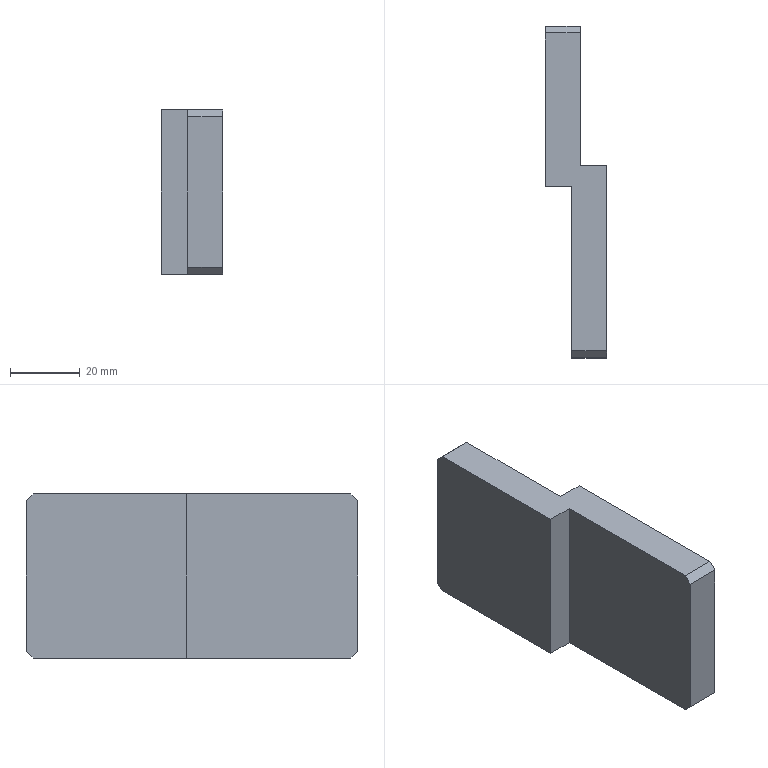Part | STEP file | PN_0041 | 1 solid | 14 faces | box 17.5 x 95 x 47 mm | volume 46685 mm3 | plane 14
STEP:
#1=CARTESIAN_POINT('',(0.,0.,0.));
#2=DIRECTION('',(0.,0.,1.));
#3=DIRECTION('',(1.,0.,0.));
#4=AXIS2_PLACEMENT_3D('',#1,#2,#3);
#5=CARTESIAN_POINT('',(10.,95.,45.));
#6=VERTEX_POINT('',#5);
#7=CARTESIAN_POINT('',(10.,95.,2.));
#8=VERTEX_POINT('',#7);
#9=CARTESIAN_POINT('',(10.,95.,47.));
#10=DIRECTION('',(0.,0.,-1.));
#11=VECTOR('',#10,1.);
#12=LINE('',#9,#11);
#13=CARTESIAN_POINT('',(0.,95.,47.));
#14=DIRECTION('',(0.,-1.,0.));
#15=DIRECTION('',(0.,0.,-1.));
#16=AXIS2_PLACEMENT_3D('',#13,#14,#15);
#17=PLANE('',#16);
#18=CARTESIAN_POINT('',(0.,10.));
#19=DIRECTION('',(1.,0.));
#20=VECTOR('',#19,1.);
#21=LINE('',#18,#20);
#22=(GEOMETRIC_REPRESENTATION_CONTEXT(2)PARAMETRIC_REPRESENTATION_CONTEXT()REPRESENTATION_CONTEXT('',''));
#23=DEFINITIONAL_REPRESENTATION('',(#21),#22);
#24=PCURVE('',#17,#23);
#25=CARTESIAN_POINT('',(10.,95.,47.));
#26=DIRECTION('',(-1.,0.,0.));
#27=DIRECTION('',(0.,-1.,0.));
#28=AXIS2_PLACEMENT_3D('',#25,#26,#27);
#29=PLANE('',#28);
#30=CARTESIAN_POINT('',(0.,0.));
#31=DIRECTION('',(0.,-1.));
#32=VECTOR('',#31,1.);
#33=LINE('',#30,#32);
#34=(GEOMETRIC_REPRESENTATION_CONTEXT(2)PARAMETRIC_REPRESENTATION_CONTEXT()REPRESENTATION_CONTEXT('',''));
#35=DEFINITIONAL_REPRESENTATION('',(#33),#34);
#36=PCURVE('',#29,#35);
#37=SURFACE_CURVE('',#12,(#24,#36),.PCURVE_S1.);
#38=EDGE_CURVE('',#6,#8,#37,.T.);
#39=ORIENTED_EDGE('',*,*,#38,.T.);
#40=CARTESIAN_POINT('',(0.,95.,2.));
#41=VERTEX_POINT('',#40);
#42=CARTESIAN_POINT('',(0.,95.,2.));
#43=DIRECTION('',(-1.,0.,0.));
#44=VECTOR('',#43,1.);
#45=LINE('',#42,#44);
#46=CARTESIAN_POINT('',(45.,0.));
#47=DIRECTION('',(0.,-1.));
#48=VECTOR('',#47,1.);
#49=LINE('',#46,#48);
#50=(GEOMETRIC_REPRESENTATION_CONTEXT(2)PARAMETRIC_REPRESENTATION_CONTEXT()REPRESENTATION_CONTEXT('',''));
#51=DEFINITIONAL_REPRESENTATION('',(#49),#50);
#52=PCURVE('',#17,#51);
#53=CARTESIAN_POINT('',(0.,95.,2.));
#54=DIRECTION('',(0.,0.7071,-0.7071));
#55=DIRECTION('',(0.,0.7071,0.7071));
#56=AXIS2_PLACEMENT_3D('',#53,#54,#55);
#57=PLANE('',#56);
#58=CARTESIAN_POINT('',(0.,0.));
#59=DIRECTION('',(0.,-1.));
#60=VECTOR('',#59,1.);
#61=LINE('',#58,#60);
#62=(GEOMETRIC_REPRESENTATION_CONTEXT(2)PARAMETRIC_REPRESENTATION_CONTEXT()REPRESENTATION_CONTEXT('',''));
#63=DEFINITIONAL_REPRESENTATION('',(#61),#62);
#64=PCURVE('',#57,#63);
#65=SURFACE_CURVE('',#45,(#52,#64),.PCURVE_S1.);
#66=EDGE_CURVE('',#8,#41,#65,.T.);
#67=ORIENTED_EDGE('',*,*,#66,.T.);
#68=CARTESIAN_POINT('',(0.,95.,45.));
#69=VERTEX_POINT('',#68);
#70=CARTESIAN_POINT('',(0.,95.,47.));
#71=DIRECTION('',(0.,0.,-1.));
#72=VECTOR('',#71,1.);
#73=LINE('',#70,#72);
#74=CARTESIAN_POINT('',(0.,0.));
#75=DIRECTION('',(1.,0.));
#76=VECTOR('',#75,1.);
#77=LINE('',#74,#76);
#78=(GEOMETRIC_REPRESENTATION_CONTEXT(2)PARAMETRIC_REPRESENTATION_CONTEXT()REPRESENTATION_CONTEXT('',''));
#79=DEFINITIONAL_REPRESENTATION('',(#77),#78);
#80=PCURVE('',#17,#79);
#81=CARTESIAN_POINT('',(0.,49.,47.));
#82=DIRECTION('',(1.,0.,0.));
#83=DIRECTION('',(0.,0.,-1.));
#84=AXIS2_PLACEMENT_3D('',#81,#82,#83);
#85=PLANE('',#84);
#86=CARTESIAN_POINT('',(0.,46.));
#87=DIRECTION('',(1.,0.));
#88=VECTOR('',#87,1.);
#89=LINE('',#86,#88);
#90=(GEOMETRIC_REPRESENTATION_CONTEXT(2)PARAMETRIC_REPRESENTATION_CONTEXT()REPRESENTATION_CONTEXT('',''));
#91=DEFINITIONAL_REPRESENTATION('',(#89),#90);
#92=PCURVE('',#85,#91);
#93=SURFACE_CURVE('',#73,(#80,#92),.PCURVE_S1.);
#94=EDGE_CURVE('',#69,#41,#93,.T.);
#95=ORIENTED_EDGE('',*,*,#94,.F.);
#96=CARTESIAN_POINT('',(0.,95.,45.));
#97=DIRECTION('',(1.,0.,0.));
#98=VECTOR('',#97,1.);
#99=LINE('',#96,#98);
#100=CARTESIAN_POINT('',(2.,0.));
#101=DIRECTION('',(0.,1.));
#102=VECTOR('',#101,1.);
#103=LINE('',#100,#102);
#104=(GEOMETRIC_REPRESENTATION_CONTEXT(2)PARAMETRIC_REPRESENTATION_CONTEXT()REPRESENTATION_CONTEXT('',''));
#105=DEFINITIONAL_REPRESENTATION('',(#103),#104);
#106=PCURVE('',#17,#105);
#107=CARTESIAN_POINT('',(10.,93.,47.));
#108=DIRECTION('',(0.,-0.7071,-0.7071));
#109=DIRECTION('',(0.,0.7071,-0.7071));
#110=AXIS2_PLACEMENT_3D('',#107,#108,#109);
#111=PLANE('',#110);
#112=CARTESIAN_POINT('',(2.828,-10.));
#113=DIRECTION('',(0.,1.));
#114=VECTOR('',#113,1.);
#115=LINE('',#112,#114);
#116=(GEOMETRIC_REPRESENTATION_CONTEXT(2)PARAMETRIC_REPRESENTATION_CONTEXT()REPRESENTATION_CONTEXT('',''));
#117=DEFINITIONAL_REPRESENTATION('',(#115),#116);
#118=PCURVE('',#111,#117);
#119=SURFACE_CURVE('',#99,(#106,#118),.PCURVE_S1.);
#120=EDGE_CURVE('',#69,#6,#119,.T.);
#121=ORIENTED_EDGE('',*,*,#120,.T.);
#122=EDGE_LOOP('',(#39,#67,#95,#121));
#123=FACE_BOUND('',#122,.T.);
#124=ADVANCED_FACE('',(#123),#17,.F.);
#125=ORIENTED_EDGE('',*,*,#94,.T.);
#126=CARTESIAN_POINT('',(0.,93.,0.));
#127=VERTEX_POINT('',#126);
#128=CARTESIAN_POINT('',(0.,95.,2.));
#129=DIRECTION('',(0.,-0.7071,-0.7071));
#130=VECTOR('',#129,1.);
#131=LINE('',#128,#130);
#132=CARTESIAN_POINT('',(45.,46.));
#133=DIRECTION('',(0.7071,-0.7071));
#134=VECTOR('',#133,1.);
#135=LINE('',#132,#134);
#136=(GEOMETRIC_REPRESENTATION_CONTEXT(2)PARAMETRIC_REPRESENTATION_CONTEXT()REPRESENTATION_CONTEXT('',''));
#137=DEFINITIONAL_REPRESENTATION('',(#135),#136);
#138=PCURVE('',#85,#137);
#139=CARTESIAN_POINT('',(0.,0.));
#140=DIRECTION('',(-1.,0.));
#141=VECTOR('',#140,1.);
#142=LINE('',#139,#141);
#143=(GEOMETRIC_REPRESENTATION_CONTEXT(2)PARAMETRIC_REPRESENTATION_CONTEXT()REPRESENTATION_CONTEXT('',''));
#144=DEFINITIONAL_REPRESENTATION('',(#142),#143);
#145=PCURVE('',#57,#144);
#146=SURFACE_CURVE('',#131,(#138,#145),.PCURVE_S1.);
#147=EDGE_CURVE('',#41,#127,#146,.T.);
#148=ORIENTED_EDGE('',*,*,#147,.T.);
#149=CARTESIAN_POINT('',(0.,49.,0.));
#150=VERTEX_POINT('',#149);
#151=CARTESIAN_POINT('',(0.,49.,0.));
#152=DIRECTION('',(0.,-1.,0.));
#153=VECTOR('',#152,1.);
#154=LINE('',#151,#153);
#155=CARTESIAN_POINT('',(47.,0.));
#156=DIRECTION('',(0.,-1.));
#157=VECTOR('',#156,1.);
#158=LINE('',#155,#157);
#159=(GEOMETRIC_REPRESENTATION_CONTEXT(2)PARAMETRIC_REPRESENTATION_CONTEXT()REPRESENTATION_CONTEXT('',''));
#160=DEFINITIONAL_REPRESENTATION('',(#158),#159);
#161=PCURVE('',#85,#160);
#162=CARTESIAN_POINT('',(10.,95.,0.));
#163=DIRECTION('',(0.,0.,-1.));
#164=DIRECTION('',(-1.,0.,0.));
#165=AXIS2_PLACEMENT_3D('',#162,#163,#164);
#166=PLANE('',#165);
#167=CARTESIAN_POINT('',(10.,-46.));
#168=DIRECTION('',(0.,-1.));
#169=VECTOR('',#168,1.);
#170=LINE('',#167,#169);
#171=(GEOMETRIC_REPRESENTATION_CONTEXT(2)PARAMETRIC_REPRESENTATION_CONTEXT()REPRESENTATION_CONTEXT('',''));
#172=DEFINITIONAL_REPRESENTATION('',(#170),#171);
#173=PCURVE('',#166,#172);
#174=SURFACE_CURVE('',#154,(#161,#173),.PCURVE_S1.);
#175=EDGE_CURVE('',#127,#150,#174,.T.);
#176=ORIENTED_EDGE('',*,*,#175,.T.);
#177=CARTESIAN_POINT('',(0.,49.,47.));
#178=VERTEX_POINT('',#177);
#179=CARTESIAN_POINT('',(0.,49.,47.));
#180=DIRECTION('',(0.,0.,-1.));
#181=VECTOR('',#180,1.);
#182=LINE('',#179,#181);
#183=CARTESIAN_POINT('',(0.,0.));
#184=DIRECTION('',(1.,0.));
#185=VECTOR('',#184,1.);
#186=LINE('',#183,#185);
#187=(GEOMETRIC_REPRESENTATION_CONTEXT(2)PARAMETRIC_REPRESENTATION_CONTEXT()REPRESENTATION_CONTEXT('',''));
#188=DEFINITIONAL_REPRESENTATION('',(#186),#187);
#189=PCURVE('',#85,#188);
#190=CARTESIAN_POINT('',(0.,49.,47.));
#191=DIRECTION('',(0.,1.,0.));
#192=DIRECTION('',(0.,0.,1.));
#193=AXIS2_PLACEMENT_3D('',#190,#191,#192);
#194=PLANE('',#193);
#195=CARTESIAN_POINT('',(0.,0.));
#196=DIRECTION('',(-1.,0.));
#197=VECTOR('',#196,1.);
#198=LINE('',#195,#197);
#199=(GEOMETRIC_REPRESENTATION_CONTEXT(2)PARAMETRIC_REPRESENTATION_CONTEXT()REPRESENTATION_CONTEXT('',''));
#200=DEFINITIONAL_REPRESENTATION('',(#198),#199);
#201=PCURVE('',#194,#200);
#202=SURFACE_CURVE('',#182,(#189,#201),.PCURVE_S1.);
#203=EDGE_CURVE('',#178,#150,#202,.T.);
#204=ORIENTED_EDGE('',*,*,#203,.F.);
#205=CARTESIAN_POINT('',(0.,93.,47.));
#206=VERTEX_POINT('',#205);
#207=CARTESIAN_POINT('',(0.,49.,47.));
#208=DIRECTION('',(0.,-1.,0.));
#209=VECTOR('',#208,1.);
#210=LINE('',#207,#209);
#211=CARTESIAN_POINT('',(0.,0.));
#212=DIRECTION('',(0.,-1.));
#213=VECTOR('',#212,1.);
#214=LINE('',#211,#213);
#215=(GEOMETRIC_REPRESENTATION_CONTEXT(2)PARAMETRIC_REPRESENTATION_CONTEXT()REPRESENTATION_CONTEXT('',''));
#216=DEFINITIONAL_REPRESENTATION('',(#214),#215);
#217=PCURVE('',#85,#216);
#218=CARTESIAN_POINT('',(10.,95.,47.));
#219=DIRECTION('',(0.,0.,-1.));
#220=DIRECTION('',(-1.,0.,0.));
#221=AXIS2_PLACEMENT_3D('',#218,#219,#220);
#222=PLANE('',#221);
#223=CARTESIAN_POINT('',(10.,-46.));
#224=DIRECTION('',(0.,-1.));
#225=VECTOR('',#224,1.);
#226=LINE('',#223,#225);
#227=(GEOMETRIC_REPRESENTATION_CONTEXT(2)PARAMETRIC_REPRESENTATION_CONTEXT()REPRESENTATION_CONTEXT('',''));
#228=DEFINITIONAL_REPRESENTATION('',(#226),#227);
#229=PCURVE('',#222,#228);
#230=SURFACE_CURVE('',#210,(#217,#229),.PCURVE_S1.);
#231=EDGE_CURVE('',#206,#178,#230,.T.);
#232=ORIENTED_EDGE('',*,*,#231,.F.);
#233=CARTESIAN_POINT('',(0.,93.,47.));
#234=DIRECTION('',(0.,0.7071,-0.7071));
#235=VECTOR('',#234,1.);
#236=LINE('',#233,#235);
#237=CARTESIAN_POINT('',(0.,44.));
#238=DIRECTION('',(0.7071,0.7071));
#239=VECTOR('',#238,1.);
#240=LINE('',#237,#239);
#241=(GEOMETRIC_REPRESENTATION_CONTEXT(2)PARAMETRIC_REPRESENTATION_CONTEXT()REPRESENTATION_CONTEXT('',''));
#242=DEFINITIONAL_REPRESENTATION('',(#240),#241);
#243=PCURVE('',#85,#242);
#244=CARTESIAN_POINT('',(0.,-10.));
#245=DIRECTION('',(1.,0.));
#246=VECTOR('',#245,1.);
#247=LINE('',#244,#246);
#248=(GEOMETRIC_REPRESENTATION_CONTEXT(2)PARAMETRIC_REPRESENTATION_CONTEXT()REPRESENTATION_CONTEXT('',''));
#249=DEFINITIONAL_REPRESENTATION('',(#247),#248);
#250=PCURVE('',#111,#249);
#251=SURFACE_CURVE('',#236,(#243,#250),.PCURVE_S1.);
#252=EDGE_CURVE('',#206,#69,#251,.T.);
#253=ORIENTED_EDGE('',*,*,#252,.T.);
#254=EDGE_LOOP('',(#125,#148,#176,#204,#232,#253));
#255=FACE_BOUND('',#254,.T.);
#256=ADVANCED_FACE('',(#255),#85,.F.);
#257=CARTESIAN_POINT('',(7.5,49.,0.));
#258=VERTEX_POINT('',#257);
#259=CARTESIAN_POINT('',(0.,49.,0.));
#260=DIRECTION('',(1.,0.,0.));
#261=VECTOR('',#260,1.);
#262=LINE('',#259,#261);
#263=CARTESIAN_POINT('',(-47.,0.));
#264=DIRECTION('',(0.,1.));
#265=VECTOR('',#264,1.);
#266=LINE('',#263,#265);
#267=(GEOMETRIC_REPRESENTATION_CONTEXT(2)PARAMETRIC_REPRESENTATION_CONTEXT()REPRESENTATION_CONTEXT('',''));
#268=DEFINITIONAL_REPRESENTATION('',(#266),#267);
#269=PCURVE('',#194,#268);
#270=CARTESIAN_POINT('',(10.,-46.));
#271=DIRECTION('',(-1.,0.));
#272=VECTOR('',#271,1.);
#273=LINE('',#270,#272);
#274=(GEOMETRIC_REPRESENTATION_CONTEXT(2)PARAMETRIC_REPRESENTATION_CONTEXT()REPRESENTATION_CONTEXT('',''));
#275=DEFINITIONAL_REPRESENTATION('',(#273),#274);
#276=PCURVE('',#166,#275);
#277=SURFACE_CURVE('',#262,(#269,#276),.PCURVE_S1.);
#278=EDGE_CURVE('',#150,#258,#277,.T.);
#279=ORIENTED_EDGE('',*,*,#278,.T.);
#280=CARTESIAN_POINT('',(7.5,49.,47.));
#281=VERTEX_POINT('',#280);
#282=CARTESIAN_POINT('',(7.5,49.,47.));
#283=DIRECTION('',(0.,0.,-1.));
#284=VECTOR('',#283,1.);
#285=LINE('',#282,#284);
#286=CARTESIAN_POINT('',(0.,7.5));
#287=DIRECTION('',(-1.,0.));
#288=VECTOR('',#287,1.);
#289=LINE('',#286,#288);
#290=(GEOMETRIC_REPRESENTATION_CONTEXT(2)PARAMETRIC_REPRESENTATION_CONTEXT()REPRESENTATION_CONTEXT('',''));
#291=DEFINITIONAL_REPRESENTATION('',(#289),#290);
#292=PCURVE('',#194,#291);
#293=CARTESIAN_POINT('',(7.5,49.,47.));
#294=DIRECTION('',(1.,0.,0.));
#295=DIRECTION('',(0.,1.,0.));
#296=AXIS2_PLACEMENT_3D('',#293,#294,#295);
#297=PLANE('',#296);
#298=CARTESIAN_POINT('',(0.,0.));
#299=DIRECTION('',(0.,-1.));
#300=VECTOR('',#299,1.);
#301=LINE('',#298,#300);
#302=(GEOMETRIC_REPRESENTATION_CONTEXT(2)PARAMETRIC_REPRESENTATION_CONTEXT()REPRESENTATION_CONTEXT('',''));
#303=DEFINITIONAL_REPRESENTATION('',(#301),#302);
#304=PCURVE('',#297,#303);
#305=SURFACE_CURVE('',#285,(#292,#304),.PCURVE_S1.);
#306=EDGE_CURVE('',#281,#258,#305,.T.);
#307=ORIENTED_EDGE('',*,*,#306,.F.);
#308=CARTESIAN_POINT('',(0.,49.,47.));
#309=DIRECTION('',(1.,0.,0.));
#310=VECTOR('',#309,1.);
#311=LINE('',#308,#310);
#312=CARTESIAN_POINT('',(0.,0.));
#313=DIRECTION('',(0.,1.));
#314=VECTOR('',#313,1.);
#315=LINE('',#312,#314);
#316=(GEOMETRIC_REPRESENTATION_CONTEXT(2)PARAMETRIC_REPRESENTATION_CONTEXT()REPRESENTATION_CONTEXT('',''));
#317=DEFINITIONAL_REPRESENTATION('',(#315),#316);
#318=PCURVE('',#194,#317);
#319=CARTESIAN_POINT('',(10.,-46.));
#320=DIRECTION('',(-1.,0.));
#321=VECTOR('',#320,1.);
#322=LINE('',#319,#321);
#323=(GEOMETRIC_REPRESENTATION_CONTEXT(2)PARAMETRIC_REPRESENTATION_CONTEXT()REPRESENTATION_CONTEXT('',''));
#324=DEFINITIONAL_REPRESENTATION('',(#322),#323);
#325=PCURVE('',#222,#324);
#326=SURFACE_CURVE('',#311,(#318,#325),.PCURVE_S1.);
#327=EDGE_CURVE('',#178,#281,#326,.T.);
#328=ORIENTED_EDGE('',*,*,#327,.F.);
#329=ORIENTED_EDGE('',*,*,#203,.T.);
#330=EDGE_LOOP('',(#279,#307,#328,#329));
#331=FACE_BOUND('',#330,.T.);
#332=ADVANCED_FACE('',(#331),#194,.F.);
#333=CARTESIAN_POINT('',(7.5,2.,0.));
#334=VERTEX_POINT('',#333);
#335=CARTESIAN_POINT('',(7.5,49.,0.));
#336=DIRECTION('',(0.,-1.,0.));
#337=VECTOR('',#336,1.);
#338=LINE('',#335,#337);
#339=CARTESIAN_POINT('',(0.,-47.));
#340=DIRECTION('',(-1.,0.));
#341=VECTOR('',#340,1.);
#342=LINE('',#339,#341);
#343=(GEOMETRIC_REPRESENTATION_CONTEXT(2)PARAMETRIC_REPRESENTATION_CONTEXT()REPRESENTATION_CONTEXT('',''));
#344=DEFINITIONAL_REPRESENTATION('',(#342),#343);
#345=PCURVE('',#297,#344);
#346=CARTESIAN_POINT('',(2.5,-46.));
#347=DIRECTION('',(0.,-1.));
#348=VECTOR('',#347,1.);
#349=LINE('',#346,#348);
#350=(GEOMETRIC_REPRESENTATION_CONTEXT(2)PARAMETRIC_REPRESENTATION_CONTEXT()REPRESENTATION_CONTEXT('',''));
#351=DEFINITIONAL_REPRESENTATION('',(#349),#350);
#352=PCURVE('',#166,#351);
#353=SURFACE_CURVE('',#338,(#345,#352),.PCURVE_S1.);
#354=EDGE_CURVE('',#258,#334,#353,.T.);
#355=ORIENTED_EDGE('',*,*,#354,.T.);
#356=CARTESIAN_POINT('',(7.5,0.,2.));
#357=VERTEX_POINT('',#356);
#358=CARTESIAN_POINT('',(7.5,0.,2.));
#359=DIRECTION('',(0.,-0.7071,0.7071));
#360=VECTOR('',#359,1.);
#361=LINE('',#358,#360);
#362=CARTESIAN_POINT('',(-49.,-45.));
#363=DIRECTION('',(-0.7071,0.7071));
#364=VECTOR('',#363,1.);
#365=LINE('',#362,#364);
#366=(GEOMETRIC_REPRESENTATION_CONTEXT(2)PARAMETRIC_REPRESENTATION_CONTEXT()REPRESENTATION_CONTEXT('',''));
#367=DEFINITIONAL_REPRESENTATION('',(#365),#366);
#368=PCURVE('',#297,#367);
#369=CARTESIAN_POINT('',(7.5,0.,2.));
#370=DIRECTION('',(0.,-0.7071,-0.7071));
#371=DIRECTION('',(0.,0.7071,-0.7071));
#372=AXIS2_PLACEMENT_3D('',#369,#370,#371);
#373=PLANE('',#372);
#374=CARTESIAN_POINT('',(0.,0.));
#375=DIRECTION('',(-1.,0.));
#376=VECTOR('',#375,1.);
#377=LINE('',#374,#376);
#378=(GEOMETRIC_REPRESENTATION_CONTEXT(2)PARAMETRIC_REPRESENTATION_CONTEXT()REPRESENTATION_CONTEXT('',''));
#379=DEFINITIONAL_REPRESENTATION('',(#377),#378);
#380=PCURVE('',#373,#379);
#381=SURFACE_CURVE('',#361,(#368,#380),.PCURVE_S1.);
#382=EDGE_CURVE('',#334,#357,#381,.T.);
#383=ORIENTED_EDGE('',*,*,#382,.T.);
#384=CARTESIAN_POINT('',(7.5,0.,45.));
#385=VERTEX_POINT('',#384);
#386=CARTESIAN_POINT('',(7.5,0.,47.));
#387=DIRECTION('',(0.,0.,-1.));
#388=VECTOR('',#387,1.);
#389=LINE('',#386,#388);
#390=CARTESIAN_POINT('',(-49.,0.));
#391=DIRECTION('',(0.,-1.));
#392=VECTOR('',#391,1.);
#393=LINE('',#390,#392);
#394=(GEOMETRIC_REPRESENTATION_CONTEXT(2)PARAMETRIC_REPRESENTATION_CONTEXT()REPRESENTATION_CONTEXT('',''));
#395=DEFINITIONAL_REPRESENTATION('',(#393),#394);
#396=PCURVE('',#297,#395);
#397=CARTESIAN_POINT('',(7.5,0.,47.));
#398=DIRECTION('',(0.,1.,0.));
#399=DIRECTION('',(0.,0.,1.));
#400=AXIS2_PLACEMENT_3D('',#397,#398,#399);
#401=PLANE('',#400);
#402=CARTESIAN_POINT('',(0.,0.));
#403=DIRECTION('',(-1.,0.));
#404=VECTOR('',#403,1.);
#405=LINE('',#402,#404);
#406=(GEOMETRIC_REPRESENTATION_CONTEXT(2)PARAMETRIC_REPRESENTATION_CONTEXT()REPRESENTATION_CONTEXT('',''));
#407=DEFINITIONAL_REPRESENTATION('',(#405),#406);
#408=PCURVE('',#401,#407);
#409=SURFACE_CURVE('',#389,(#396,#408),.PCURVE_S1.);
#410=EDGE_CURVE('',#385,#357,#409,.T.);
#411=ORIENTED_EDGE('',*,*,#410,.F.);
#412=CARTESIAN_POINT('',(7.5,2.,47.));
#413=VERTEX_POINT('',#412);
#414=CARTESIAN_POINT('',(7.5,2.,47.));
#415=DIRECTION('',(0.,0.7071,0.7071));
#416=VECTOR('',#415,1.);
#417=LINE('',#414,#416);
#418=CARTESIAN_POINT('',(-47.,0.));
#419=DIRECTION('',(0.7071,0.7071));
#420=VECTOR('',#419,1.);
#421=LINE('',#418,#420);
#422=(GEOMETRIC_REPRESENTATION_CONTEXT(2)PARAMETRIC_REPRESENTATION_CONTEXT()REPRESENTATION_CONTEXT('',''));
#423=DEFINITIONAL_REPRESENTATION('',(#421),#422);
#424=PCURVE('',#297,#423);
#425=CARTESIAN_POINT('',(10.,2.,47.));
#426=DIRECTION('',(0.,0.7071,-0.7071));
#427=DIRECTION('',(0.,0.7071,0.7071));
#428=AXIS2_PLACEMENT_3D('',#425,#426,#427);
#429=PLANE('',#428);
#430=CARTESIAN_POINT('',(0.,-2.5));
#431=DIRECTION('',(1.,0.));
#432=VECTOR('',#431,1.);
#433=LINE('',#430,#432);
#434=(GEOMETRIC_REPRESENTATION_CONTEXT(2)PARAMETRIC_REPRESENTATION_CONTEXT()REPRESENTATION_CONTEXT('',''));
#435=DEFINITIONAL_REPRESENTATION('',(#433),#434);
#436=PCURVE('',#429,#435);
#437=SURFACE_CURVE('',#417,(#424,#436),.PCURVE_S1.);
#438=EDGE_CURVE('',#385,#413,#437,.T.);
#439=ORIENTED_EDGE('',*,*,#438,.T.);
#440=CARTESIAN_POINT('',(7.5,49.,47.));
#441=DIRECTION('',(0.,-1.,0.));
#442=VECTOR('',#441,1.);
#443=LINE('',#440,#442);
#444=CARTESIAN_POINT('',(0.,0.));
#445=DIRECTION('',(-1.,0.));
#446=VECTOR('',#445,1.);
#447=LINE('',#444,#446);
#448=(GEOMETRIC_REPRESENTATION_CONTEXT(2)PARAMETRIC_REPRESENTATION_CONTEXT()REPRESENTATION_CONTEXT('',''));
#449=DEFINITIONAL_REPRESENTATION('',(#447),#448);
#450=PCURVE('',#297,#449);
#451=CARTESIAN_POINT('',(2.5,-46.));
#452=DIRECTION('',(0.,-1.));
#453=VECTOR('',#452,1.);
#454=LINE('',#451,#453);
#455=(GEOMETRIC_REPRESENTATION_CONTEXT(2)PARAMETRIC_REPRESENTATION_CONTEXT()REPRESENTATION_CONTEXT('',''));
#456=DEFINITIONAL_REPRESENTATION('',(#454),#455);
#457=PCURVE('',#222,#456);
#458=SURFACE_CURVE('',#443,(#450,#457),.PCURVE_S1.);
#459=EDGE_CURVE('',#281,#413,#458,.T.);
#460=ORIENTED_EDGE('',*,*,#459,.F.);
#461=ORIENTED_EDGE('',*,*,#306,.T.);
#462=EDGE_LOOP('',(#355,#383,#411,#439,#460,#461));
#463=FACE_BOUND('',#462,.T.);
#464=ADVANCED_FACE('',(#463),#297,.F.);
#465=ORIENTED_EDGE('',*,*,#410,.T.);
#466=CARTESIAN_POINT('',(17.5,0.,2.));
#467=VERTEX_POINT('',#466);
#468=CARTESIAN_POINT('',(17.5,0.,2.));
#469=DIRECTION('',(1.,0.,0.));
#470=VECTOR('',#469,1.);
#471=LINE('',#468,#470);
#472=CARTESIAN_POINT('',(-45.,10.));
#473=DIRECTION('',(0.,1.));
#474=VECTOR('',#473,1.);
#475=LINE('',#472,#474);
#476=(GEOMETRIC_REPRESENTATION_CONTEXT(2)PARAMETRIC_REPRESENTATION_CONTEXT()REPRESENTATION_CONTEXT('',''));
#477=DEFINITIONAL_REPRESENTATION('',(#475),#476);
#478=PCURVE('',#401,#477);
#479=CARTESIAN_POINT('',(0.,10.));
#480=DIRECTION('',(0.,1.));
#481=VECTOR('',#480,1.);
#482=LINE('',#479,#481);
#483=(GEOMETRIC_REPRESENTATION_CONTEXT(2)PARAMETRIC_REPRESENTATION_CONTEXT()REPRESENTATION_CONTEXT('',''));
#484=DEFINITIONAL_REPRESENTATION('',(#482),#483);
#485=PCURVE('',#373,#484);
#486=SURFACE_CURVE('',#471,(#478,#485),.PCURVE_S1.);
#487=EDGE_CURVE('',#357,#467,#486,.T.);
#488=ORIENTED_EDGE('',*,*,#487,.T.);
#489=CARTESIAN_POINT('',(17.5,0.,45.));
#490=VERTEX_POINT('',#489);
#491=CARTESIAN_POINT('',(17.5,0.,47.));
#492=DIRECTION('',(0.,0.,-1.));
#493=VECTOR('',#492,1.);
#494=LINE('',#491,#493);
#495=CARTESIAN_POINT('',(0.,10.));
#496=DIRECTION('',(-1.,0.));
#497=VECTOR('',#496,1.);
#498=LINE('',#495,#497);
#499=(GEOMETRIC_REPRESENTATION_CONTEXT(2)PARAMETRIC_REPRESENTATION_CONTEXT()REPRESENTATION_CONTEXT('',''));
#500=DEFINITIONAL_REPRESENTATION('',(#498),#499);
#501=PCURVE('',#401,#500);
#502=CARTESIAN_POINT('',(17.5,0.,47.));
#503=DIRECTION('',(-1.,0.,0.));
#504=DIRECTION('',(0.,0.,1.));
#505=AXIS2_PLACEMENT_3D('',#502,#503,#504);
#506=PLANE('',#505);
#507=CARTESIAN_POINT('',(0.,0.));
#508=DIRECTION('',(-1.,0.));
#509=VECTOR('',#508,1.);
#510=LINE('',#507,#509);
#511=(GEOMETRIC_REPRESENTATION_CONTEXT(2)PARAMETRIC_REPRESENTATION_CONTEXT()REPRESENTATION_CONTEXT('',''));
#512=DEFINITIONAL_REPRESENTATION('',(#510),#511);
#513=PCURVE('',#506,#512);
#514=SURFACE_CURVE('',#494,(#501,#513),.PCURVE_S1.);
#515=EDGE_CURVE('',#490,#467,#514,.T.);
#516=ORIENTED_EDGE('',*,*,#515,.F.);
#517=CARTESIAN_POINT('',(7.5,0.,45.));
#518=DIRECTION('',(-1.,0.,0.));
#519=VECTOR('',#518,1.);
#520=LINE('',#517,#519);
#521=CARTESIAN_POINT('',(-2.,0.));
#522=DIRECTION('',(0.,-1.));
#523=VECTOR('',#522,1.);
#524=LINE('',#521,#523);
#525=(GEOMETRIC_REPRESENTATION_CONTEXT(2)PARAMETRIC_REPRESENTATION_CONTEXT()REPRESENTATION_CONTEXT('',''));
#526=DEFINITIONAL_REPRESENTATION('',(#524),#525);
#527=PCURVE('',#401,#526);
#528=CARTESIAN_POINT('',(-2.828,-2.5));
#529=DIRECTION('',(0.,-1.));
#530=VECTOR('',#529,1.);
#531=LINE('',#528,#530);
#532=(GEOMETRIC_REPRESENTATION_CONTEXT(2)PARAMETRIC_REPRESENTATION_CONTEXT()REPRESENTATION_CONTEXT('',''));
#533=DEFINITIONAL_REPRESENTATION('',(#531),#532);
#534=PCURVE('',#429,#533);
#535=SURFACE_CURVE('',#520,(#527,#534),.PCURVE_S1.);
#536=EDGE_CURVE('',#490,#385,#535,.T.);
#537=ORIENTED_EDGE('',*,*,#536,.T.);
#538=EDGE_LOOP('',(#465,#488,#516,#537));
#539=FACE_BOUND('',#538,.T.);
#540=ADVANCED_FACE('',(#539),#401,.F.);
#541=ORIENTED_EDGE('',*,*,#515,.T.);
#542=CARTESIAN_POINT('',(17.5,2.,0.));
#543=VERTEX_POINT('',#542);
#544=CARTESIAN_POINT('',(17.5,0.,2.));
#545=DIRECTION('',(0.,0.7071,-0.7071));
#546=VECTOR('',#545,1.);
#547=LINE('',#544,#546);
#548=CARTESIAN_POINT('',(-45.,0.));
#549=DIRECTION('',(-0.7071,0.7071));
#550=VECTOR('',#549,1.);
#551=LINE('',#548,#550);
#552=(GEOMETRIC_REPRESENTATION_CONTEXT(2)PARAMETRIC_REPRESENTATION_CONTEXT()REPRESENTATION_CONTEXT('',''));
#553=DEFINITIONAL_REPRESENTATION('',(#551),#552);
#554=PCURVE('',#506,#553);
#555=CARTESIAN_POINT('',(0.,10.));
#556=DIRECTION('',(1.,0.));
#557=VECTOR('',#556,1.);
#558=LINE('',#555,#557);
#559=(GEOMETRIC_REPRESENTATION_CONTEXT(2)PARAMETRIC_REPRESENTATION_CONTEXT()REPRESENTATION_CONTEXT('',''));
#560=DEFINITIONAL_REPRESENTATION('',(#558),#559);
#561=PCURVE('',#373,#560);
#562=SURFACE_CURVE('',#547,(#554,#561),.PCURVE_S1.);
#563=EDGE_CURVE('',#467,#543,#562,.T.);
#564=ORIENTED_EDGE('',*,*,#563,.T.);
#565=CARTESIAN_POINT('',(17.5,55.,0.));
#566=VERTEX_POINT('',#565);
#567=CARTESIAN_POINT('',(17.5,0.,0.));
#568=DIRECTION('',(0.,1.,0.));
#569=VECTOR('',#568,1.);
#570=LINE('',#567,#569);
#571=CARTESIAN_POINT('',(-47.,0.));
#572=DIRECTION('',(0.,1.));
#573=VECTOR('',#572,1.);
#574=LINE('',#571,#573);
#575=(GEOMETRIC_REPRESENTATION_CONTEXT(2)PARAMETRIC_REPRESENTATION_CONTEXT()REPRESENTATION_CONTEXT('',''));
#576=DEFINITIONAL_REPRESENTATION('',(#574),#575);
#577=PCURVE('',#506,#576);
#578=CARTESIAN_POINT('',(-7.5,-95.));
#579=DIRECTION('',(0.,1.));
#580=VECTOR('',#579,1.);
#581=LINE('',#578,#580);
#582=(GEOMETRIC_REPRESENTATION_CONTEXT(2)PARAMETRIC_REPRESENTATION_CONTEXT()REPRESENTATION_CONTEXT('',''));
#583=DEFINITIONAL_REPRESENTATION('',(#581),#582);
#584=PCURVE('',#166,#583);
#585=SURFACE_CURVE('',#570,(#577,#584),.PCURVE_S1.);
#586=EDGE_CURVE('',#543,#566,#585,.T.);
#587=ORIENTED_EDGE('',*,*,#586,.T.);
#588=CARTESIAN_POINT('',(17.5,55.,47.));
#589=VERTEX_POINT('',#588);
#590=CARTESIAN_POINT('',(17.5,55.,47.));
#591=DIRECTION('',(0.,0.,-1.));
#592=VECTOR('',#591,1.);
#593=LINE('',#590,#592);
#594=CARTESIAN_POINT('',(0.,55.));
#595=DIRECTION('',(-1.,0.));
#596=VECTOR('',#595,1.);
#597=LINE('',#594,#596);
#598=(GEOMETRIC_REPRESENTATION_CONTEXT(2)PARAMETRIC_REPRESENTATION_CONTEXT()REPRESENTATION_CONTEXT('',''));
#599=DEFINITIONAL_REPRESENTATION('',(#597),#598);
#600=PCURVE('',#506,#599);
#601=CARTESIAN_POINT('',(10.,55.,47.));
#602=DIRECTION('',(0.,-1.,0.));
#603=DIRECTION('',(0.,0.,-1.));
#604=AXIS2_PLACEMENT_3D('',#601,#602,#603);
#605=PLANE('',#604);
#606=CARTESIAN_POINT('',(0.,7.5));
#607=DIRECTION('',(1.,0.));
#608=VECTOR('',#607,1.);
#609=LINE('',#606,#608);
#610=(GEOMETRIC_REPRESENTATION_CONTEXT(2)PARAMETRIC_REPRESENTATION_CONTEXT()REPRESENTATION_CONTEXT('',''));
#611=DEFINITIONAL_REPRESENTATION('',(#609),#610);
#612=PCURVE('',#605,#611);
#613=SURFACE_CURVE('',#593,(#600,#612),.PCURVE_S1.);
#614=EDGE_CURVE('',#589,#566,#613,.T.);
#615=ORIENTED_EDGE('',*,*,#614,.F.);
#616=CARTESIAN_POINT('',(17.5,2.,47.));
#617=VERTEX_POINT('',#616);
#618=CARTESIAN_POINT('',(17.5,0.,47.));
#619=DIRECTION('',(0.,1.,0.));
#620=VECTOR('',#619,1.);
#621=LINE('',#618,#620);
#622=CARTESIAN_POINT('',(0.,0.));
#623=DIRECTION('',(0.,1.));
#624=VECTOR('',#623,1.);
#625=LINE('',#622,#624);
#626=(GEOMETRIC_REPRESENTATION_CONTEXT(2)PARAMETRIC_REPRESENTATION_CONTEXT()REPRESENTATION_CONTEXT('',''));
#627=DEFINITIONAL_REPRESENTATION('',(#625),#626);
#628=PCURVE('',#506,#627);
#629=CARTESIAN_POINT('',(-7.5,-95.));
#630=DIRECTION('',(0.,1.));
#631=VECTOR('',#630,1.);
#632=LINE('',#629,#631);
#633=(GEOMETRIC_REPRESENTATION_CONTEXT(2)PARAMETRIC_REPRESENTATION_CONTEXT()REPRESENTATION_CONTEXT('',''));
#634=DEFINITIONAL_REPRESENTATION('',(#632),#633);
#635=PCURVE('',#222,#634);
#636=SURFACE_CURVE('',#621,(#628,#635),.PCURVE_S1.);
#637=EDGE_CURVE('',#617,#589,#636,.T.);
#638=ORIENTED_EDGE('',*,*,#637,.F.);
#639=CARTESIAN_POINT('',(17.5,2.,47.));
#640=DIRECTION('',(0.,-0.7071,-0.7071));
#641=VECTOR('',#640,1.);
#642=LINE('',#639,#641);
#643=CARTESIAN_POINT('',(0.,2.));
#644=DIRECTION('',(-0.7071,-0.7071));
#645=VECTOR('',#644,1.);
#646=LINE('',#643,#645);
#647=(GEOMETRIC_REPRESENTATION_CONTEXT(2)PARAMETRIC_REPRESENTATION_CONTEXT()REPRESENTATION_CONTEXT('',''));
#648=DEFINITIONAL_REPRESENTATION('',(#646),#647);
#649=PCURVE('',#506,#648);
#650=CARTESIAN_POINT('',(0.,7.5));
#651=DIRECTION('',(-1.,0.));
#652=VECTOR('',#651,1.);
#653=LINE('',#650,#652);
#654=(GEOMETRIC_REPRESENTATION_CONTEXT(2)PARAMETRIC_REPRESENTATION_CONTEXT()REPRESENTATION_CONTEXT('',''));
#655=DEFINITIONAL_REPRESENTATION('',(#653),#654);
#656=PCURVE('',#429,#655);
#657=SURFACE_CURVE('',#642,(#649,#656),.PCURVE_S1.);
#658=EDGE_CURVE('',#617,#490,#657,.T.);
#659=ORIENTED_EDGE('',*,*,#658,.T.);
#660=EDGE_LOOP('',(#541,#564,#587,#615,#638,#659));
#661=FACE_BOUND('',#660,.T.);
#662=ADVANCED_FACE('',(#661),#506,.F.);
#663=CARTESIAN_POINT('',(10.,55.,0.));
#664=VERTEX_POINT('',#663);
#665=CARTESIAN_POINT('',(10.,55.,0.));
#666=DIRECTION('',(-1.,0.,0.));
#667=VECTOR('',#666,1.);
#668=LINE('',#665,#667);
#669=CARTESIAN_POINT('',(47.,0.));
#670=DIRECTION('',(0.,-1.));
#671=VECTOR('',#670,1.);
#672=LINE('',#669,#671);
#673=(GEOMETRIC_REPRESENTATION_CONTEXT(2)PARAMETRIC_REPRESENTATION_CONTEXT()REPRESENTATION_CONTEXT('',''));
#674=DEFINITIONAL_REPRESENTATION('',(#672),#673);
#675=PCURVE('',#605,#674);
#676=CARTESIAN_POINT('',(0.,-40.));
#677=DIRECTION('',(1.,0.));
#678=VECTOR('',#677,1.);
#679=LINE('',#676,#678);
#680=(GEOMETRIC_REPRESENTATION_CONTEXT(2)PARAMETRIC_REPRESENTATION_CONTEXT()REPRESENTATION_CONTEXT('',''));
#681=DEFINITIONAL_REPRESENTATION('',(#679),#680);
#682=PCURVE('',#166,#681);
#683=SURFACE_CURVE('',#668,(#675,#682),.PCURVE_S1.);
#684=EDGE_CURVE('',#566,#664,#683,.T.);
#685=ORIENTED_EDGE('',*,*,#684,.T.);
#686=CARTESIAN_POINT('',(10.,55.,47.));
#687=VERTEX_POINT('',#686);
#688=CARTESIAN_POINT('',(10.,55.,47.));
#689=DIRECTION('',(0.,0.,-1.));
#690=VECTOR('',#689,1.);
#691=LINE('',#688,#690);
#692=CARTESIAN_POINT('',(0.,0.));
#693=DIRECTION('',(1.,0.));
#694=VECTOR('',#693,1.);
#695=LINE('',#692,#694);
#696=(GEOMETRIC_REPRESENTATION_CONTEXT(2)PARAMETRIC_REPRESENTATION_CONTEXT()REPRESENTATION_CONTEXT('',''));
#697=DEFINITIONAL_REPRESENTATION('',(#695),#696);
#698=PCURVE('',#605,#697);
#699=CARTESIAN_POINT('',(40.,0.));
#700=DIRECTION('',(0.,-1.));
#701=VECTOR('',#700,1.);
#702=LINE('',#699,#701);
#703=(GEOMETRIC_REPRESENTATION_CONTEXT(2)PARAMETRIC_REPRESENTATION_CONTEXT()REPRESENTATION_CONTEXT('',''));
#704=DEFINITIONAL_REPRESENTATION('',(#702),#703);
#705=PCURVE('',#29,#704);
#706=SURFACE_CURVE('',#691,(#698,#705),.PCURVE_S1.);
#707=EDGE_CURVE('',#687,#664,#706,.T.);
#708=ORIENTED_EDGE('',*,*,#707,.F.);
#709=CARTESIAN_POINT('',(10.,55.,47.));
#710=DIRECTION('',(-1.,0.,0.));
#711=VECTOR('',#710,1.);
#712=LINE('',#709,#711);
#713=CARTESIAN_POINT('',(0.,0.));
#714=DIRECTION('',(0.,-1.));
#715=VECTOR('',#714,1.);
#716=LINE('',#713,#715);
#717=(GEOMETRIC_REPRESENTATION_CONTEXT(2)PARAMETRIC_REPRESENTATION_CONTEXT()REPRESENTATION_CONTEXT('',''));
#718=DEFINITIONAL_REPRESENTATION('',(#716),#717);
#719=PCURVE('',#605,#718);
#720=CARTESIAN_POINT('',(0.,-40.));
#721=DIRECTION('',(1.,0.));
#722=VECTOR('',#721,1.);
#723=LINE('',#720,#722);
#724=(GEOMETRIC_REPRESENTATION_CONTEXT(2)PARAMETRIC_REPRESENTATION_CONTEXT()REPRESENTATION_CONTEXT('',''));
#725=DEFINITIONAL_REPRESENTATION('',(#723),#724);
#726=PCURVE('',#222,#725);
#727=SURFACE_CURVE('',#712,(#719,#726),.PCURVE_S1.);
#728=EDGE_CURVE('',#589,#687,#727,.T.);
#729=ORIENTED_EDGE('',*,*,#728,.F.);
#730=ORIENTED_EDGE('',*,*,#614,.T.);
#731=EDGE_LOOP('',(#685,#708,#729,#730));
#732=FACE_BOUND('',#731,.T.);
#733=ADVANCED_FACE('',(#732),#605,.F.);
#734=CARTESIAN_POINT('',(10.,93.,0.));
#735=VERTEX_POINT('',#734);
#736=CARTESIAN_POINT('',(10.,95.,0.));
#737=DIRECTION('',(0.,1.,0.));
#738=VECTOR('',#737,1.);
#739=LINE('',#736,#738);
#740=CARTESIAN_POINT('',(0.,-47.));
#741=DIRECTION('',(-1.,0.));
#742=VECTOR('',#741,1.);
#743=LINE('',#740,#742);
#744=(GEOMETRIC_REPRESENTATION_CONTEXT(2)PARAMETRIC_REPRESENTATION_CONTEXT()REPRESENTATION_CONTEXT('',''));
#745=DEFINITIONAL_REPRESENTATION('',(#743),#744);
#746=PCURVE('',#29,#745);
#747=CARTESIAN_POINT('',(0.,0.));
#748=DIRECTION('',(0.,1.));
#749=VECTOR('',#748,1.);
#750=LINE('',#747,#749);
#751=(GEOMETRIC_REPRESENTATION_CONTEXT(2)PARAMETRIC_REPRESENTATION_CONTEXT()REPRESENTATION_CONTEXT('',''));
#752=DEFINITIONAL_REPRESENTATION('',(#750),#751);
#753=PCURVE('',#166,#752);
#754=SURFACE_CURVE('',#739,(#746,#753),.PCURVE_S1.);
#755=EDGE_CURVE('',#664,#735,#754,.T.);
#756=ORIENTED_EDGE('',*,*,#755,.T.);
#757=CARTESIAN_POINT('',(10.,95.,2.));
#758=DIRECTION('',(0.,0.7071,0.7071));
#759=VECTOR('',#758,1.);
#760=LINE('',#757,#759);
#761=CARTESIAN_POINT('',(0.,-45.));
#762=DIRECTION('',(-0.7071,0.7071));
#763=VECTOR('',#762,1.);
#764=LINE('',#761,#763);
#765=(GEOMETRIC_REPRESENTATION_CONTEXT(2)PARAMETRIC_REPRESENTATION_CONTEXT()REPRESENTATION_CONTEXT('',''));
#766=DEFINITIONAL_REPRESENTATION('',(#764),#765);
#767=PCURVE('',#29,#766);
#768=CARTESIAN_POINT('',(0.,10.));
#769=DIRECTION('',(1.,0.));
#770=VECTOR('',#769,1.);
#771=LINE('',#768,#770);
#772=(GEOMETRIC_REPRESENTATION_CONTEXT(2)PARAMETRIC_REPRESENTATION_CONTEXT()REPRESENTATION_CONTEXT('',''));
#773=DEFINITIONAL_REPRESENTATION('',(#771),#772);
#774=PCURVE('',#57,#773);
#775=SURFACE_CURVE('',#760,(#767,#774),.PCURVE_S1.);
#776=EDGE_CURVE('',#735,#8,#775,.T.);
#777=ORIENTED_EDGE('',*,*,#776,.T.);
#778=ORIENTED_EDGE('',*,*,#38,.F.);
#779=CARTESIAN_POINT('',(10.,93.,47.));
#780=VERTEX_POINT('',#779);
#781=CARTESIAN_POINT('',(10.,93.,47.));
#782=DIRECTION('',(0.,-0.7071,0.7071));
#783=VECTOR('',#782,1.);
#784=LINE('',#781,#783);
#785=CARTESIAN_POINT('',(2.,0.));
#786=DIRECTION('',(0.7071,0.7071));
#787=VECTOR('',#786,1.);
#788=LINE('',#785,#787);
#789=(GEOMETRIC_REPRESENTATION_CONTEXT(2)PARAMETRIC_REPRESENTATION_CONTEXT()REPRESENTATION_CONTEXT('',''));
#790=DEFINITIONAL_REPRESENTATION('',(#788),#789);
#791=PCURVE('',#29,#790);
#792=CARTESIAN_POINT('',(0.,0.));
#793=DIRECTION('',(-1.,0.));
#794=VECTOR('',#793,1.);
#795=LINE('',#792,#794);
#796=(GEOMETRIC_REPRESENTATION_CONTEXT(2)PARAMETRIC_REPRESENTATION_CONTEXT()REPRESENTATION_CONTEXT('',''));
#797=DEFINITIONAL_REPRESENTATION('',(#795),#796);
#798=PCURVE('',#111,#797);
#799=SURFACE_CURVE('',#784,(#791,#798),.PCURVE_S1.);
#800=EDGE_CURVE('',#6,#780,#799,.T.);
#801=ORIENTED_EDGE('',*,*,#800,.T.);
#802=CARTESIAN_POINT('',(10.,95.,47.));
#803=DIRECTION('',(0.,1.,0.));
#804=VECTOR('',#803,1.);
#805=LINE('',#802,#804);
#806=CARTESIAN_POINT('',(0.,0.));
#807=DIRECTION('',(-1.,0.));
#808=VECTOR('',#807,1.);
#809=LINE('',#806,#808);
#810=(GEOMETRIC_REPRESENTATION_CONTEXT(2)PARAMETRIC_REPRESENTATION_CONTEXT()REPRESENTATION_CONTEXT('',''));
#811=DEFINITIONAL_REPRESENTATION('',(#809),#810);
#812=PCURVE('',#29,#811);
#813=CARTESIAN_POINT('',(0.,0.));
#814=DIRECTION('',(0.,1.));
#815=VECTOR('',#814,1.);
#816=LINE('',#813,#815);
#817=(GEOMETRIC_REPRESENTATION_CONTEXT(2)PARAMETRIC_REPRESENTATION_CONTEXT()REPRESENTATION_CONTEXT('',''));
#818=DEFINITIONAL_REPRESENTATION('',(#816),#817);
#819=PCURVE('',#222,#818);
#820=SURFACE_CURVE('',#805,(#812,#819),.PCURVE_S1.);
#821=EDGE_CURVE('',#687,#780,#820,.T.);
#822=ORIENTED_EDGE('',*,*,#821,.F.);
#823=ORIENTED_EDGE('',*,*,#707,.T.);
#824=EDGE_LOOP('',(#756,#777,#778,#801,#822,#823));
#825=FACE_BOUND('',#824,.T.);
#826=ADVANCED_FACE('',(#825),#29,.F.);
#827=ORIENTED_EDGE('',*,*,#459,.T.);
#828=CARTESIAN_POINT('',(10.,2.,47.));
#829=DIRECTION('',(1.,0.,0.));
#830=VECTOR('',#829,1.);
#831=LINE('',#828,#830);
#832=CARTESIAN_POINT('',(0.,-93.));
#833=DIRECTION('',(-1.,0.));
#834=VECTOR('',#833,1.);
#835=LINE('',#832,#834);
#836=(GEOMETRIC_REPRESENTATION_CONTEXT(2)PARAMETRIC_REPRESENTATION_CONTEXT()REPRESENTATION_CONTEXT('',''));
#837=DEFINITIONAL_REPRESENTATION('',(#835),#836);
#838=PCURVE('',#222,#837);
#839=CARTESIAN_POINT('',(0.,0.));
#840=DIRECTION('',(0.,1.));
#841=VECTOR('',#840,1.);
#842=LINE('',#839,#841);
#843=(GEOMETRIC_REPRESENTATION_CONTEXT(2)PARAMETRIC_REPRESENTATION_CONTEXT()REPRESENTATION_CONTEXT('',''));
#844=DEFINITIONAL_REPRESENTATION('',(#842),#843);
#845=PCURVE('',#429,#844);
#846=SURFACE_CURVE('',#831,(#838,#845),.PCURVE_S1.);
#847=EDGE_CURVE('',#413,#617,#846,.T.);
#848=ORIENTED_EDGE('',*,*,#847,.T.);
#849=ORIENTED_EDGE('',*,*,#637,.T.);
#850=ORIENTED_EDGE('',*,*,#728,.T.);
#851=ORIENTED_EDGE('',*,*,#821,.T.);
#852=CARTESIAN_POINT('',(10.,93.,47.));
#853=DIRECTION('',(-1.,0.,0.));
#854=VECTOR('',#853,1.);
#855=LINE('',#852,#854);
#856=CARTESIAN_POINT('',(0.,-2.));
#857=DIRECTION('',(1.,0.));
#858=VECTOR('',#857,1.);
#859=LINE('',#856,#858);
#860=(GEOMETRIC_REPRESENTATION_CONTEXT(2)PARAMETRIC_REPRESENTATION_CONTEXT()REPRESENTATION_CONTEXT('',''));
#861=DEFINITIONAL_REPRESENTATION('',(#859),#860);
#862=PCURVE('',#222,#861);
#863=CARTESIAN_POINT('',(0.,0.));
#864=DIRECTION('',(0.,-1.));
#865=VECTOR('',#864,1.);
#866=LINE('',#863,#865);
#867=(GEOMETRIC_REPRESENTATION_CONTEXT(2)PARAMETRIC_REPRESENTATION_CONTEXT()REPRESENTATION_CONTEXT('',''));
#868=DEFINITIONAL_REPRESENTATION('',(#866),#867);
#869=PCURVE('',#111,#868);
#870=SURFACE_CURVE('',#855,(#862,#869),.PCURVE_S1.);
#871=EDGE_CURVE('',#780,#206,#870,.T.);
#872=ORIENTED_EDGE('',*,*,#871,.T.);
#873=ORIENTED_EDGE('',*,*,#231,.T.);
#874=ORIENTED_EDGE('',*,*,#327,.T.);
#875=EDGE_LOOP('',(#827,#848,#849,#850,#851,#872,#873,#874));
#876=FACE_BOUND('',#875,.T.);
#877=ADVANCED_FACE('',(#876),#222,.F.);
#878=ORIENTED_EDGE('',*,*,#586,.F.);
#879=CARTESIAN_POINT('',(7.5,2.,0.));
#880=DIRECTION('',(-1.,0.,0.));
#881=VECTOR('',#880,1.);
#882=LINE('',#879,#881);
#883=CARTESIAN_POINT('',(2.5,-93.));
#884=DIRECTION('',(1.,0.));
#885=VECTOR('',#884,1.);
#886=LINE('',#883,#885);
#887=(GEOMETRIC_REPRESENTATION_CONTEXT(2)PARAMETRIC_REPRESENTATION_CONTEXT()REPRESENTATION_CONTEXT('',''));
#888=DEFINITIONAL_REPRESENTATION('',(#886),#887);
#889=PCURVE('',#166,#888);
#890=CARTESIAN_POINT('',(2.828,0.));
#891=DIRECTION('',(0.,-1.));
#892=VECTOR('',#891,1.);
#893=LINE('',#890,#892);
#894=(GEOMETRIC_REPRESENTATION_CONTEXT(2)PARAMETRIC_REPRESENTATION_CONTEXT()REPRESENTATION_CONTEXT('',''));
#895=DEFINITIONAL_REPRESENTATION('',(#893),#894);
#896=PCURVE('',#373,#895);
#897=SURFACE_CURVE('',#882,(#889,#896),.PCURVE_S1.);
#898=EDGE_CURVE('',#543,#334,#897,.T.);
#899=ORIENTED_EDGE('',*,*,#898,.T.);
#900=ORIENTED_EDGE('',*,*,#354,.F.);
#901=ORIENTED_EDGE('',*,*,#278,.F.);
#902=ORIENTED_EDGE('',*,*,#175,.F.);
#903=CARTESIAN_POINT('',(10.,93.,0.));
#904=DIRECTION('',(1.,0.,0.));
#905=VECTOR('',#904,1.);
#906=LINE('',#903,#905);
#907=CARTESIAN_POINT('',(0.,-2.));
#908=DIRECTION('',(-1.,0.));
#909=VECTOR('',#908,1.);
#910=LINE('',#907,#909);
#911=(GEOMETRIC_REPRESENTATION_CONTEXT(2)PARAMETRIC_REPRESENTATION_CONTEXT()REPRESENTATION_CONTEXT('',''));
#912=DEFINITIONAL_REPRESENTATION('',(#910),#911);
#913=PCURVE('',#166,#912);
#914=CARTESIAN_POINT('',(-2.828,10.));
#915=DIRECTION('',(0.,1.));
#916=VECTOR('',#915,1.);
#917=LINE('',#914,#916);
#918=(GEOMETRIC_REPRESENTATION_CONTEXT(2)PARAMETRIC_REPRESENTATION_CONTEXT()REPRESENTATION_CONTEXT('',''));
#919=DEFINITIONAL_REPRESENTATION('',(#917),#918);
#920=PCURVE('',#57,#919);
#921=SURFACE_CURVE('',#906,(#913,#920),.PCURVE_S1.);
#922=EDGE_CURVE('',#127,#735,#921,.T.);
#923=ORIENTED_EDGE('',*,*,#922,.T.);
#924=ORIENTED_EDGE('',*,*,#755,.F.);
#925=ORIENTED_EDGE('',*,*,#684,.F.);
#926=EDGE_LOOP('',(#878,#899,#900,#901,#902,#923,#924,#925));
#927=FACE_BOUND('',#926,.T.);
#928=ADVANCED_FACE('',(#927),#166,.T.);
#929=ORIENTED_EDGE('',*,*,#382,.F.);
#930=ORIENTED_EDGE('',*,*,#898,.F.);
#931=ORIENTED_EDGE('',*,*,#563,.F.);
#932=ORIENTED_EDGE('',*,*,#487,.F.);
#933=EDGE_LOOP('',(#929,#930,#931,#932));
#934=FACE_BOUND('',#933,.T.);
#935=ADVANCED_FACE('',(#934),#373,.T.);
#936=ORIENTED_EDGE('',*,*,#438,.F.);
#937=ORIENTED_EDGE('',*,*,#536,.F.);
#938=ORIENTED_EDGE('',*,*,#658,.F.);
#939=ORIENTED_EDGE('',*,*,#847,.F.);
#940=EDGE_LOOP('',(#936,#937,#938,#939));
#941=FACE_BOUND('',#940,.T.);
#942=ADVANCED_FACE('',(#941),#429,.F.);
#943=ORIENTED_EDGE('',*,*,#776,.F.);
#944=ORIENTED_EDGE('',*,*,#922,.F.);
#945=ORIENTED_EDGE('',*,*,#147,.F.);
#946=ORIENTED_EDGE('',*,*,#66,.F.);
#947=EDGE_LOOP('',(#943,#944,#945,#946));
#948=FACE_BOUND('',#947,.T.);
#949=ADVANCED_FACE('',(#948),#57,.T.);
#950=ORIENTED_EDGE('',*,*,#800,.F.);
#951=ORIENTED_EDGE('',*,*,#120,.F.);
#952=ORIENTED_EDGE('',*,*,#252,.F.);
#953=ORIENTED_EDGE('',*,*,#871,.F.);
#954=EDGE_LOOP('',(#950,#951,#952,#953));
#955=FACE_BOUND('',#954,.T.);
#956=ADVANCED_FACE('',(#955),#111,.F.);
#957=CLOSED_SHELL('',(#124,#256,#332,#464,#540,#662,#733,#826,#877,#928,#935,#942,#949,#956));
#958=MANIFOLD_SOLID_BREP('',#957);
#959=(LENGTH_UNIT()NAMED_UNIT(*)SI_UNIT(.MILLI.,.METRE.));
#960=UNCERTAINTY_MEASURE_WITH_UNIT(LENGTH_MEASURE(0.0000001),#959,'','');
#961=(NAMED_UNIT(*)PLANE_ANGLE_UNIT()SI_UNIT($,.RADIAN.));
#962=(NAMED_UNIT(*)SI_UNIT($,.STERADIAN.)SOLID_ANGLE_UNIT());
#963=(GEOMETRIC_REPRESENTATION_CONTEXT(3)GLOBAL_UNCERTAINTY_ASSIGNED_CONTEXT((#960))GLOBAL_UNIT_ASSIGNED_CONTEXT((#959,#961,#962))REPRESENTATION_CONTEXT('',''));
#964=ADVANCED_BREP_SHAPE_REPRESENTATION('',(#4,#958),#963);